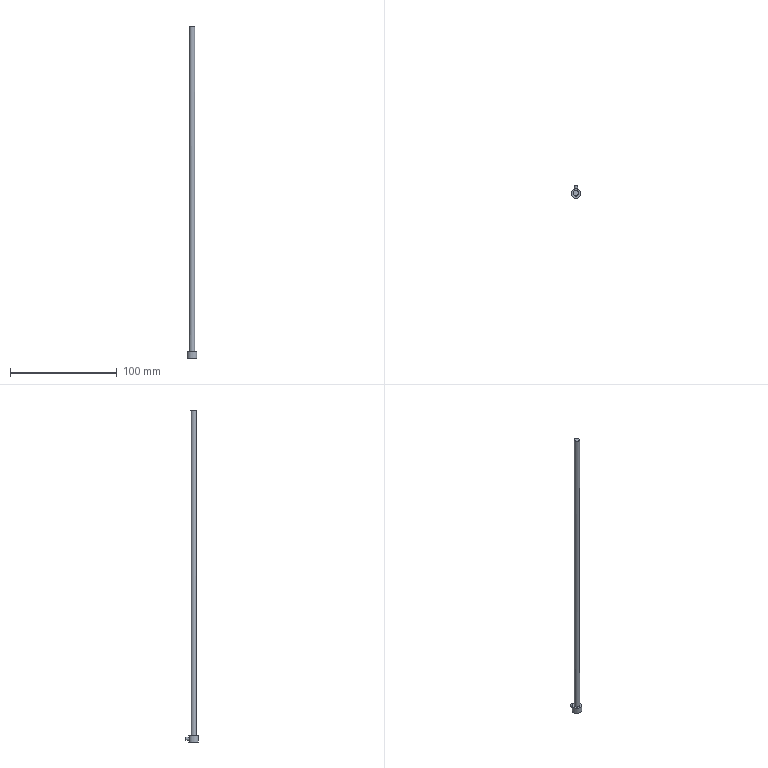Part | STEP file | E105-29-315 | 1 solid | 8 faces | box 9 x 12 x 311.151 mm | volume 6392 mm3 | cylinder 3 | plane 3 | spline 1 | cone 1 | commonest cylinder face diameters 3 x1 5 x1 9 x1
STEP:
#1=CARTESIAN_POINT('',(0.,0.,0.));
#2=DIRECTION('',(0.,0.,1.));
#3=DIRECTION('',(1.,0.,0.));
#4=AXIS2_PLACEMENT_3D('',#1,#2,#3);
#5=CARTESIAN_POINT('',(2.494,-0.1722,310.881));
#6=VERTEX_POINT('',#5);
#7=CARTESIAN_POINT('',(-2.5,0.,311.113));
#8=VERTEX_POINT('',#7);
#9=CARTESIAN_POINT('',(2.494,-0.1722,310.881));
#10=CARTESIAN_POINT('',(2.475,-0.4516,310.892));
#11=CARTESIAN_POINT('',(2.407,-0.7315,310.907));
#12=CARTESIAN_POINT('',(2.296,-0.9886,310.923));
#13=CARTESIAN_POINT('',(2.186,-1.246,310.939));
#14=CARTESIAN_POINT('',(2.029,-1.487,310.957));
#15=CARTESIAN_POINT('',(1.839,-1.693,310.975));
#16=CARTESIAN_POINT('',(1.65,-1.899,310.994));
#17=CARTESIAN_POINT('',(1.422,-2.075,311.013));
#18=CARTESIAN_POINT('',(1.174,-2.207,311.031));
#19=CARTESIAN_POINT('',(0.9268,-2.339,311.049));
#20=CARTESIAN_POINT('',(0.653,-2.429,311.066));
#21=CARTESIAN_POINT('',(0.3756,-2.472,311.081));
#22=CARTESIAN_POINT('',(0.09849,-2.514,311.097));
#23=CARTESIAN_POINT('',(-0.1899,-2.509,311.11));
#24=CARTESIAN_POINT('',(-0.4655,-2.456,311.121));
#25=CARTESIAN_POINT('',(-0.7405,-2.404,311.131));
#26=CARTESIAN_POINT('',(-1.01,-2.304,311.14));
#27=CARTESIAN_POINT('',(-1.253,-2.163,311.145));
#28=CARTESIAN_POINT('',(-1.495,-2.023,311.15));
#29=CARTESIAN_POINT('',(-1.716,-1.84,311.152));
#30=CARTESIAN_POINT('',(-1.898,-1.627,311.151));
#31=CARTESIAN_POINT('',(-2.08,-1.415,311.15));
#32=CARTESIAN_POINT('',(-2.227,-1.169,311.147));
#33=CARTESIAN_POINT('',(-2.329,-0.909,311.141));
#34=CARTESIAN_POINT('',(-2.43,-0.6487,311.135));
#35=CARTESIAN_POINT('',(-2.489,-0.3675,311.126));
#36=CARTESIAN_POINT('',(-2.498,-0.08843,311.116));
#37=CARTESIAN_POINT('',(-2.508,0.191,311.106));
#38=CARTESIAN_POINT('',(-2.47,0.4758,311.094));
#39=CARTESIAN_POINT('',(-2.387,0.7427,311.08));
#40=CARTESIAN_POINT('',(-2.304,1.01,311.067));
#41=CARTESIAN_POINT('',(-2.174,1.266,311.052));
#42=CARTESIAN_POINT('',(-2.007,1.491,311.037));
#43=CARTESIAN_POINT('',(-1.84,1.716,311.022));
#44=CARTESIAN_POINT('',(-1.632,1.915,311.006));
#45=CARTESIAN_POINT('',(-1.4,2.072,310.99));
#46=CARTESIAN_POINT('',(-1.167,2.228,310.974));
#47=CARTESIAN_POINT('',(-0.9049,2.347,310.958));
#48=CARTESIAN_POINT('',(-0.6337,2.418,310.943));
#49=CARTESIAN_POINT('',(-0.3626,2.489,310.928));
#50=CARTESIAN_POINT('',(-0.07546,2.515,310.914));
#51=CARTESIAN_POINT('',(0.204,2.492,310.901));
#52=CARTESIAN_POINT('',(0.4832,2.469,310.889));
#53=CARTESIAN_POINT('',(0.7624,2.397,310.877));
#54=CARTESIAN_POINT('',(1.018,2.283,310.868));
#55=CARTESIAN_POINT('',(1.274,2.169,310.859));
#56=CARTESIAN_POINT('',(1.514,2.009,310.853));
#57=CARTESIAN_POINT('',(1.717,1.817,310.849));
#58=CARTESIAN_POINT('',(1.92,1.625,310.845));
#59=CARTESIAN_POINT('',(2.093,1.395,310.844));
#60=CARTESIAN_POINT('',(2.221,1.147,310.846));
#61=CARTESIAN_POINT('',(2.349,0.8988,310.848));
#62=CARTESIAN_POINT('',(2.437,0.6252,310.854));
#63=CARTESIAN_POINT('',(2.476,0.3488,310.862));
#64=CARTESIAN_POINT('',(2.5,0.1767,310.867));
#65=CARTESIAN_POINT('',(2.506,0.001161,310.873));
#66=CARTESIAN_POINT('',(2.494,-0.1722,310.881));
#67=B_SPLINE_CURVE_WITH_KNOTS('',3,(#9,#10,#11,#12,#13,#14,#15,#16,#17,#18,#19,#20,#21,#22,#23,#24,#25,#26,#27,#28,#29,#30,#31,#32,#33,#34,#35,#36,#37,#38,#39,#40,#41,#42,#43,#44,#45,#46,#47,#48,#49,#50,#51,#52,#53,#54,#55,#56,#57,#58,#59,#60,#61,#62,#63,#64,#65,#66),.UNSPECIFIED.,.T.,.F.,(1,3,3,3,3,3,3,3,3,3,3,3,3,3,3,3,3,3,3,3,3,1),(-0.03305,0.,0.05377,0.1075,0.1614,0.2153,0.2691,0.3228,0.3764,0.43,0.4835,0.5372,0.5909,0.6447,0.6985,0.7523,0.8061,0.8598,0.9134,0.967,1.,1.054),.UNSPECIFIED.);
#68=CARTESIAN_POINT('',(0.,0.,106.));
#69=DIRECTION('',(0.,0.,-1.));
#70=DIRECTION('',(-1.,0.,0.));
#71=AXIS2_PLACEMENT_3D('',#68,#69,#70);
#72=CYLINDRICAL_SURFACE('',#71,2.5);
#73=CARTESIAN_POINT('',(3.211,-204.881));
#74=CARTESIAN_POINT('',(3.234,-204.883));
#75=CARTESIAN_POINT('',(3.282,-204.888));
#76=CARTESIAN_POINT('',(3.353,-204.897));
#77=CARTESIAN_POINT('',(3.425,-204.906));
#78=CARTESIAN_POINT('',(3.496,-204.916));
#79=CARTESIAN_POINT('',(3.567,-204.926));
#80=CARTESIAN_POINT('',(3.638,-204.936));
#81=CARTESIAN_POINT('',(3.71,-204.947));
#82=CARTESIAN_POINT('',(3.781,-204.958));
#83=CARTESIAN_POINT('',(3.853,-204.97));
#84=CARTESIAN_POINT('',(3.924,-204.981));
#85=CARTESIAN_POINT('',(3.995,-204.993));
#86=CARTESIAN_POINT('',(4.067,-205.005));
#87=CARTESIAN_POINT('',(4.138,-205.017));
#88=CARTESIAN_POINT('',(4.209,-205.028));
#89=CARTESIAN_POINT('',(4.28,-205.04));
#90=CARTESIAN_POINT('',(4.352,-205.051));
#91=CARTESIAN_POINT('',(4.423,-205.062));
#92=CARTESIAN_POINT('',(4.495,-205.072));
#93=CARTESIAN_POINT('',(4.566,-205.082));
#94=CARTESIAN_POINT('',(4.637,-205.091));
#95=CARTESIAN_POINT('',(4.708,-205.1));
#96=CARTESIAN_POINT('',(4.78,-205.108));
#97=CARTESIAN_POINT('',(4.851,-205.116));
#98=CARTESIAN_POINT('',(4.922,-205.123));
#99=CARTESIAN_POINT('',(4.994,-205.129));
#100=CARTESIAN_POINT('',(5.065,-205.135));
#101=CARTESIAN_POINT('',(5.137,-205.139));
#102=CARTESIAN_POINT('',(5.208,-205.143));
#103=CARTESIAN_POINT('',(5.279,-205.147));
#104=CARTESIAN_POINT('',(5.351,-205.149));
#105=CARTESIAN_POINT('',(5.423,-205.151));
#106=CARTESIAN_POINT('',(5.494,-205.151));
#107=CARTESIAN_POINT('',(5.566,-205.151));
#108=CARTESIAN_POINT('',(5.637,-205.151));
#109=CARTESIAN_POINT('',(5.708,-205.149));
#110=CARTESIAN_POINT('',(5.78,-205.147));
#111=CARTESIAN_POINT('',(5.852,-205.144));
#112=CARTESIAN_POINT('',(5.923,-205.14));
#113=CARTESIAN_POINT('',(5.994,-205.136));
#114=CARTESIAN_POINT('',(6.066,-205.131));
#115=CARTESIAN_POINT('',(6.137,-205.126));
#116=CARTESIAN_POINT('',(6.209,-205.12));
#117=CARTESIAN_POINT('',(6.28,-205.113));
#118=CARTESIAN_POINT('',(6.351,-205.106));
#119=CARTESIAN_POINT('',(6.423,-205.099));
#120=CARTESIAN_POINT('',(6.494,-205.091));
#121=CARTESIAN_POINT('',(6.566,-205.083));
#122=CARTESIAN_POINT('',(6.637,-205.074));
#123=CARTESIAN_POINT('',(6.708,-205.065));
#124=CARTESIAN_POINT('',(6.78,-205.056));
#125=CARTESIAN_POINT('',(6.851,-205.047));
#126=CARTESIAN_POINT('',(6.922,-205.037));
#127=CARTESIAN_POINT('',(6.993,-205.027));
#128=CARTESIAN_POINT('',(7.065,-205.017));
#129=CARTESIAN_POINT('',(7.136,-205.007));
#130=CARTESIAN_POINT('',(7.208,-204.997));
#131=CARTESIAN_POINT('',(7.279,-204.987));
#132=CARTESIAN_POINT('',(7.35,-204.977));
#133=CARTESIAN_POINT('',(7.422,-204.967));
#134=CARTESIAN_POINT('',(7.493,-204.958));
#135=CARTESIAN_POINT('',(7.564,-204.948));
#136=CARTESIAN_POINT('',(7.635,-204.938));
#137=CARTESIAN_POINT('',(7.707,-204.929));
#138=CARTESIAN_POINT('',(7.778,-204.92));
#139=CARTESIAN_POINT('',(7.85,-204.911));
#140=CARTESIAN_POINT('',(7.921,-204.903));
#141=CARTESIAN_POINT('',(7.992,-204.895));
#142=CARTESIAN_POINT('',(8.064,-204.887));
#143=CARTESIAN_POINT('',(8.135,-204.88));
#144=CARTESIAN_POINT('',(8.207,-204.874));
#145=CARTESIAN_POINT('',(8.278,-204.868));
#146=CARTESIAN_POINT('',(8.349,-204.863));
#147=CARTESIAN_POINT('',(8.421,-204.858));
#148=CARTESIAN_POINT('',(8.492,-204.854));
#149=CARTESIAN_POINT('',(8.564,-204.85));
#150=CARTESIAN_POINT('',(8.635,-204.848));
#151=CARTESIAN_POINT('',(8.706,-204.846));
#152=CARTESIAN_POINT('',(8.778,-204.845));
#153=CARTESIAN_POINT('',(8.85,-204.845));
#154=CARTESIAN_POINT('',(8.921,-204.846));
#155=CARTESIAN_POINT('',(8.992,-204.847));
#156=CARTESIAN_POINT('',(9.064,-204.849));
#157=CARTESIAN_POINT('',(9.135,-204.853));
#158=CARTESIAN_POINT('',(9.207,-204.857));
#159=CARTESIAN_POINT('',(9.278,-204.861));
#160=CARTESIAN_POINT('',(9.35,-204.867));
#161=CARTESIAN_POINT('',(9.422,-204.873));
#162=CARTESIAN_POINT('',(9.47,-204.878));
#163=CARTESIAN_POINT('',(9.494,-204.881));
#164=B_SPLINE_CURVE_WITH_KNOTS('',3,(#73,#74,#75,#76,#77,#78,#79,#80,#81,#82,#83,#84,#85,#86,#87,#88,#89,#90,#91,#92,#93,#94,#95,#96,#97,#98,#99,#100,#101,#102,#103,#104,#105,#106,#107,#108,#109,#110,#111,#112,#113,#114,#115,#116,#117,#118,#119,#120,#121,#122,#123,#124,#125,#126,#127,#128,#129,#130,#131,#132,#133,#134,#135,#136,#137,#138,#139,#140,#141,#142,#143,#144,#145,#146,#147,#148,#149,#150,#151,#152,#153,#154,#155,#156,#157,#158,#159,#160,#161,#162,#163),.UNSPECIFIED.,.F.,.F.,(4,1,1,1,1,1,1,1,1,1,1,1,1,1,1,1,1,1,1,1,1,1,1,1,1,1,1,1,1,1,1,1,1,1,1,1,1,1,1,1,1,1,1,1,1,1,1,1,1,1,1,1,1,1,1,1,1,1,1,1,1,1,1,1,1,1,1,1,1,1,1,1,1,1,1,1,1,1,1,1,1,1,1,1,1,1,1,1,4),(0.,0.01136,0.02273,0.03409,0.04545,0.05682,0.06818,0.07955,0.09091,0.1023,0.1136,0.125,0.1364,0.1477,0.1591,0.1705,0.1818,0.1932,0.2045,0.2159,0.2273,0.2386,0.25,0.2614,0.2727,0.2841,0.2955,0.3068,0.3182,0.3295,0.3409,0.3523,0.3636,0.375,0.3864,0.3977,0.4091,0.4205,0.4318,0.4432,0.4545,0.4659,0.4773,0.4886,0.5,0.5114,0.5227,0.5341,0.5455,0.5568,0.5682,0.5795,0.5909,0.6023,0.6136,0.625,0.6364,0.6477,0.6591,0.6705,0.6818,0.6932,0.7045,0.7159,0.7273,0.7386,0.75,0.7614,0.7727,0.7841,0.7955,0.8068,0.8182,0.8295,0.8409,0.8523,0.8636,0.875,0.8864,0.8977,0.9091,0.9205,0.9318,0.9432,0.9545,0.9659,0.9773,0.9886,1.),.QUASI_UNIFORM_KNOTS.);
#165=(GEOMETRIC_REPRESENTATION_CONTEXT(2)PARAMETRIC_REPRESENTATION_CONTEXT()REPRESENTATION_CONTEXT('',''));
#166=DEFINITIONAL_REPRESENTATION('',(#164),#165);
#167=PCURVE('',#72,#166);
#168=CARTESIAN_POINT('',(-12.782,-3.331,311.416));
#169=CARTESIAN_POINT('',(-7.05,-3.329,311.438));
#170=CARTESIAN_POINT('',(-1.256,-3.327,311.257));
#171=CARTESIAN_POINT('',(4.609,-3.325,310.869));
#172=CARTESIAN_POINT('',(-12.796,-0.9979,311.327));
#173=CARTESIAN_POINT('',(-7.066,-0.9958,311.349));
#174=CARTESIAN_POINT('',(-1.274,-0.9937,311.169));
#175=CARTESIAN_POINT('',(4.59,-0.9916,310.782));
#176=CARTESIAN_POINT('',(-12.81,1.335,311.238));
#177=CARTESIAN_POINT('',(-7.082,1.337,311.261));
#178=CARTESIAN_POINT('',(-1.292,1.339,311.081));
#179=CARTESIAN_POINT('',(4.57,1.342,310.695));
#180=CARTESIAN_POINT('',(-12.825,3.668,311.148));
#181=CARTESIAN_POINT('',(-7.099,3.671,311.172));
#182=CARTESIAN_POINT('',(-1.31,3.673,310.993));
#183=CARTESIAN_POINT('',(4.55,3.675,310.608));
#184=B_SPLINE_SURFACE_WITH_KNOTS('',3,3,((#168,#169,#170,#171),(#172,#173,#174,#175),(#176,#177,#178,#179),(#180,#181,#182,#183)),.UNSPECIFIED.,.F.,.F.,.F.,(4,4),(4,4),(0.,1.),(0.,1.),.PIECEWISE_BEZIER_KNOTS.);
#185=CARTESIAN_POINT('',(0.4505,0.8811));
#186=CARTESIAN_POINT('',(0.4423,0.8808));
#187=CARTESIAN_POINT('',(0.4257,0.8801));
#188=CARTESIAN_POINT('',(0.4011,0.8783));
#189=CARTESIAN_POINT('',(0.3768,0.8758));
#190=CARTESIAN_POINT('',(0.3531,0.8726));
#191=CARTESIAN_POINT('',(0.33,0.8689));
#192=CARTESIAN_POINT('',(0.3077,0.8644));
#193=CARTESIAN_POINT('',(0.286,0.8594));
#194=CARTESIAN_POINT('',(0.2653,0.8537));
#195=CARTESIAN_POINT('',(0.2456,0.8475));
#196=CARTESIAN_POINT('',(0.2271,0.8409));
#197=CARTESIAN_POINT('',(0.2098,0.8337));
#198=CARTESIAN_POINT('',(0.1938,0.826));
#199=CARTESIAN_POINT('',(0.1791,0.8179));
#200=CARTESIAN_POINT('',(0.1658,0.8094));
#201=CARTESIAN_POINT('',(0.1541,0.8006));
#202=CARTESIAN_POINT('',(0.144,0.7914));
#203=CARTESIAN_POINT('',(0.1354,0.782));
#204=CARTESIAN_POINT('',(0.1285,0.7724));
#205=CARTESIAN_POINT('',(0.1233,0.7626));
#206=CARTESIAN_POINT('',(0.1198,0.7528));
#207=CARTESIAN_POINT('',(0.118,0.7428));
#208=CARTESIAN_POINT('',(0.118,0.7328));
#209=CARTESIAN_POINT('',(0.1197,0.7228));
#210=CARTESIAN_POINT('',(0.1231,0.7129));
#211=CARTESIAN_POINT('',(0.1283,0.7032));
#212=CARTESIAN_POINT('',(0.1352,0.6936));
#213=CARTESIAN_POINT('',(0.1437,0.6842));
#214=CARTESIAN_POINT('',(0.1539,0.675));
#215=CARTESIAN_POINT('',(0.1655,0.6663));
#216=CARTESIAN_POINT('',(0.1787,0.6578));
#217=CARTESIAN_POINT('',(0.1934,0.6497));
#218=CARTESIAN_POINT('',(0.2095,0.6421));
#219=CARTESIAN_POINT('',(0.2269,0.6349));
#220=CARTESIAN_POINT('',(0.2454,0.6283));
#221=CARTESIAN_POINT('',(0.265,0.6222));
#222=CARTESIAN_POINT('',(0.2858,0.6166));
#223=CARTESIAN_POINT('',(0.3075,0.6116));
#224=CARTESIAN_POINT('',(0.3299,0.6073));
#225=CARTESIAN_POINT('',(0.353,0.6036));
#226=CARTESIAN_POINT('',(0.3767,0.6006));
#227=CARTESIAN_POINT('',(0.401,0.5982));
#228=CARTESIAN_POINT('',(0.4257,0.5966));
#229=CARTESIAN_POINT('',(0.4505,0.5956));
#230=CARTESIAN_POINT('',(0.4671,0.5954));
#231=CARTESIAN_POINT('',(0.4754,0.5954));
#232=B_SPLINE_CURVE_WITH_KNOTS('',3,(#185,#186,#187,#188,#189,#190,#191,#192,#193,#194,#195,#196,#197,#198,#199,#200,#201,#202,#203,#204,#205,#206,#207,#208,#209,#210,#211,#212,#213,#214,#215,#216,#217,#218,#219,#220,#221,#222,#223,#224,#225,#226,#227,#228,#229,#230,#231),.UNSPECIFIED.,.F.,.F.,(4,1,1,1,1,1,1,1,1,1,1,1,1,1,1,1,1,1,1,1,1,1,1,1,1,1,1,1,1,1,1,1,1,1,1,1,1,1,1,1,1,1,1,1,4),(0.,0.01112,0.02224,0.03335,0.04447,0.05559,0.06671,0.07783,0.08894,0.1001,0.1112,0.1223,0.1334,0.1445,0.1557,0.1668,0.1779,0.189,0.2001,0.2112,0.2224,0.2335,0.2446,0.2557,0.2668,0.2779,0.2891,0.3002,0.3113,0.3224,0.3335,0.3447,0.3558,0.3669,0.378,0.3891,0.4002,0.4114,0.4225,0.4336,0.4447,0.4558,0.467,0.4781,0.4892),.QUASI_UNIFORM_KNOTS.);
#233=(GEOMETRIC_REPRESENTATION_CONTEXT(2)PARAMETRIC_REPRESENTATION_CONTEXT()REPRESENTATION_CONTEXT('',''));
#234=DEFINITIONAL_REPRESENTATION('',(#232),#233);
#235=PCURVE('',#184,#234);
#236=SURFACE_CURVE('',#67,(#167,#235),.PCURVE_S1.);
#237=EDGE_CURVE('',#6,#8,#236,.T.);
#238=ORIENTED_EDGE('',*,*,#237,.T.);
#239=CARTESIAN_POINT('',(-2.5,0.,6.));
#240=VERTEX_POINT('',#239);
#241=CARTESIAN_POINT('',(-2.5,0.,311.113));
#242=CARTESIAN_POINT('',(-2.5,0.,6.));
#243=B_SPLINE_CURVE_WITH_KNOTS('',1,(#241,#242),.UNSPECIFIED.,.F.,.F.,(2,2),(-205.113,100.),.PIECEWISE_BEZIER_KNOTS.);
#244=CARTESIAN_POINT('',(6.283,0.));
#245=DIRECTION('',(0.,1.));
#246=VECTOR('',#245,1.);
#247=LINE('',#244,#246);
#248=(GEOMETRIC_REPRESENTATION_CONTEXT(2)PARAMETRIC_REPRESENTATION_CONTEXT()REPRESENTATION_CONTEXT('',''));
#249=DEFINITIONAL_REPRESENTATION('',(#247),#248);
#250=PCURVE('',#72,#249);
#251=CARTESIAN_POINT('',(0.,0.));
#252=DIRECTION('',(0.,1.));
#253=VECTOR('',#252,1.);
#254=LINE('',#251,#253);
#255=(GEOMETRIC_REPRESENTATION_CONTEXT(2)PARAMETRIC_REPRESENTATION_CONTEXT()REPRESENTATION_CONTEXT('',''));
#256=DEFINITIONAL_REPRESENTATION('',(#254),#255);
#257=PCURVE('',#72,#256);
#258=SEAM_CURVE('',#243,(#250,#257),.PCURVE_S1.);
#259=EDGE_CURVE('',#8,#240,#258,.T.);
#260=ORIENTED_EDGE('',*,*,#259,.T.);
#261=CARTESIAN_POINT('',(0.,0.,6.));
#262=DIRECTION('',(0.,0.,-1.));
#263=DIRECTION('',(-1.,0.,0.));
#264=AXIS2_PLACEMENT_3D('',#261,#262,#263);
#265=CIRCLE('',#264,2.5);
#266=CARTESIAN_POINT('',(0.,100.));
#267=DIRECTION('',(1.,0.));
#268=VECTOR('',#267,1.);
#269=LINE('',#266,#268);
#270=(GEOMETRIC_REPRESENTATION_CONTEXT(2)PARAMETRIC_REPRESENTATION_CONTEXT()REPRESENTATION_CONTEXT('',''));
#271=DEFINITIONAL_REPRESENTATION('',(#269),#270);
#272=PCURVE('',#72,#271);
#273=CARTESIAN_POINT('',(0.,0.,6.));
#274=DIRECTION('',(0.,0.,-1.));
#275=DIRECTION('',(1.,0.,0.));
#276=AXIS2_PLACEMENT_3D('',#273,#274,#275);
#277=PLANE('',#276);
#278=CARTESIAN_POINT('',(0.,0.));
#279=DIRECTION('',(-1.,0.));
#280=AXIS2_PLACEMENT_2D('',#278,#279);
#281=CIRCLE('',#280,2.5);
#282=(GEOMETRIC_REPRESENTATION_CONTEXT(2)PARAMETRIC_REPRESENTATION_CONTEXT()REPRESENTATION_CONTEXT('',''));
#283=DEFINITIONAL_REPRESENTATION('',(#281),#282);
#284=PCURVE('',#277,#283);
#285=SURFACE_CURVE('',#265,(#272,#284),.PCURVE_S1.);
#286=EDGE_CURVE('',#240,#240,#285,.T.);
#287=ORIENTED_EDGE('',*,*,#286,.F.);
#288=ORIENTED_EDGE('',*,*,#259,.F.);
#289=CARTESIAN_POINT('',(2.494,-0.1722,310.881));
#290=CARTESIAN_POINT('',(2.475,-0.4516,310.892));
#291=CARTESIAN_POINT('',(2.407,-0.7315,310.907));
#292=CARTESIAN_POINT('',(2.296,-0.9886,310.923));
#293=CARTESIAN_POINT('',(2.186,-1.246,310.939));
#294=CARTESIAN_POINT('',(2.029,-1.487,310.957));
#295=CARTESIAN_POINT('',(1.839,-1.693,310.975));
#296=CARTESIAN_POINT('',(1.65,-1.899,310.994));
#297=CARTESIAN_POINT('',(1.422,-2.075,311.013));
#298=CARTESIAN_POINT('',(1.174,-2.207,311.031));
#299=CARTESIAN_POINT('',(0.9268,-2.339,311.049));
#300=CARTESIAN_POINT('',(0.653,-2.429,311.066));
#301=CARTESIAN_POINT('',(0.3756,-2.472,311.081));
#302=CARTESIAN_POINT('',(0.09849,-2.514,311.097));
#303=CARTESIAN_POINT('',(-0.1899,-2.509,311.11));
#304=CARTESIAN_POINT('',(-0.4655,-2.456,311.121));
#305=CARTESIAN_POINT('',(-0.7405,-2.404,311.131));
#306=CARTESIAN_POINT('',(-1.01,-2.304,311.14));
#307=CARTESIAN_POINT('',(-1.253,-2.163,311.145));
#308=CARTESIAN_POINT('',(-1.495,-2.023,311.15));
#309=CARTESIAN_POINT('',(-1.716,-1.84,311.152));
#310=CARTESIAN_POINT('',(-1.898,-1.627,311.151));
#311=CARTESIAN_POINT('',(-2.08,-1.415,311.15));
#312=CARTESIAN_POINT('',(-2.227,-1.169,311.147));
#313=CARTESIAN_POINT('',(-2.329,-0.909,311.141));
#314=CARTESIAN_POINT('',(-2.43,-0.6487,311.135));
#315=CARTESIAN_POINT('',(-2.489,-0.3675,311.126));
#316=CARTESIAN_POINT('',(-2.498,-0.08843,311.116));
#317=CARTESIAN_POINT('',(-2.508,0.191,311.106));
#318=CARTESIAN_POINT('',(-2.47,0.4758,311.094));
#319=CARTESIAN_POINT('',(-2.387,0.7427,311.08));
#320=CARTESIAN_POINT('',(-2.304,1.01,311.067));
#321=CARTESIAN_POINT('',(-2.174,1.266,311.052));
#322=CARTESIAN_POINT('',(-2.007,1.491,311.037));
#323=CARTESIAN_POINT('',(-1.84,1.716,311.022));
#324=CARTESIAN_POINT('',(-1.632,1.915,311.006));
#325=CARTESIAN_POINT('',(-1.4,2.072,310.99));
#326=CARTESIAN_POINT('',(-1.167,2.228,310.974));
#327=CARTESIAN_POINT('',(-0.9049,2.347,310.958));
#328=CARTESIAN_POINT('',(-0.6337,2.418,310.943));
#329=CARTESIAN_POINT('',(-0.3626,2.489,310.928));
#330=CARTESIAN_POINT('',(-0.07546,2.515,310.914));
#331=CARTESIAN_POINT('',(0.204,2.492,310.901));
#332=CARTESIAN_POINT('',(0.4832,2.469,310.889));
#333=CARTESIAN_POINT('',(0.7624,2.397,310.877));
#334=CARTESIAN_POINT('',(1.018,2.283,310.868));
#335=CARTESIAN_POINT('',(1.274,2.169,310.859));
#336=CARTESIAN_POINT('',(1.514,2.009,310.853));
#337=CARTESIAN_POINT('',(1.717,1.817,310.849));
#338=CARTESIAN_POINT('',(1.92,1.625,310.845));
#339=CARTESIAN_POINT('',(2.093,1.395,310.844));
#340=CARTESIAN_POINT('',(2.221,1.147,310.846));
#341=CARTESIAN_POINT('',(2.349,0.8988,310.848));
#342=CARTESIAN_POINT('',(2.437,0.6252,310.854));
#343=CARTESIAN_POINT('',(2.476,0.3488,310.862));
#344=CARTESIAN_POINT('',(2.5,0.1767,310.867));
#345=CARTESIAN_POINT('',(2.506,0.001161,310.873));
#346=CARTESIAN_POINT('',(2.494,-0.1722,310.881));
#347=B_SPLINE_CURVE_WITH_KNOTS('',3,(#289,#290,#291,#292,#293,#294,#295,#296,#297,#298,#299,#300,#301,#302,#303,#304,#305,#306,#307,#308,#309,#310,#311,#312,#313,#314,#315,#316,#317,#318,#319,#320,#321,#322,#323,#324,#325,#326,#327,#328,#329,#330,#331,#332,#333,#334,#335,#336,#337,#338,#339,#340,#341,#342,#343,#344,#345,#346),.UNSPECIFIED.,.T.,.F.,(1,3,3,3,3,3,3,3,3,3,3,3,3,3,3,3,3,3,3,3,3,1),(-0.03305,0.,0.05377,0.1075,0.1614,0.2153,0.2691,0.3228,0.3764,0.43,0.4835,0.5372,0.5909,0.6447,0.6985,0.7523,0.8061,0.8598,0.9134,0.967,1.,1.054),.UNSPECIFIED.);
#348=CARTESIAN_POINT('',(-3.073,-204.881));
#349=CARTESIAN_POINT('',(-3.049,-204.883));
#350=CARTESIAN_POINT('',(-3.001,-204.888));
#351=CARTESIAN_POINT('',(-2.93,-204.897));
#352=CARTESIAN_POINT('',(-2.858,-204.906));
#353=CARTESIAN_POINT('',(-2.787,-204.916));
#354=CARTESIAN_POINT('',(-2.716,-204.926));
#355=CARTESIAN_POINT('',(-2.645,-204.936));
#356=CARTESIAN_POINT('',(-2.573,-204.947));
#357=CARTESIAN_POINT('',(-2.502,-204.958));
#358=CARTESIAN_POINT('',(-2.43,-204.97));
#359=CARTESIAN_POINT('',(-2.359,-204.981));
#360=CARTESIAN_POINT('',(-2.288,-204.993));
#361=CARTESIAN_POINT('',(-2.217,-205.005));
#362=CARTESIAN_POINT('',(-2.145,-205.017));
#363=CARTESIAN_POINT('',(-2.074,-205.028));
#364=CARTESIAN_POINT('',(-2.003,-205.04));
#365=CARTESIAN_POINT('',(-1.932,-205.051));
#366=CARTESIAN_POINT('',(-1.86,-205.062));
#367=CARTESIAN_POINT('',(-1.789,-205.072));
#368=CARTESIAN_POINT('',(-1.718,-205.082));
#369=CARTESIAN_POINT('',(-1.646,-205.091));
#370=CARTESIAN_POINT('',(-1.575,-205.1));
#371=CARTESIAN_POINT('',(-1.503,-205.108));
#372=CARTESIAN_POINT('',(-1.432,-205.116));
#373=CARTESIAN_POINT('',(-1.361,-205.123));
#374=CARTESIAN_POINT('',(-1.289,-205.129));
#375=CARTESIAN_POINT('',(-1.218,-205.135));
#376=CARTESIAN_POINT('',(-1.146,-205.139));
#377=CARTESIAN_POINT('',(-1.075,-205.143));
#378=CARTESIAN_POINT('',(-1.004,-205.147));
#379=CARTESIAN_POINT('',(-0.9322,-205.149));
#380=CARTESIAN_POINT('',(-0.8606,-205.151));
#381=CARTESIAN_POINT('',(-0.7889,-205.151));
#382=CARTESIAN_POINT('',(-0.7176,-205.151));
#383=CARTESIAN_POINT('',(-0.6465,-205.151));
#384=CARTESIAN_POINT('',(-0.5749,-205.149));
#385=CARTESIAN_POINT('',(-0.5033,-205.147));
#386=CARTESIAN_POINT('',(-0.4317,-205.144));
#387=CARTESIAN_POINT('',(-0.3605,-205.14));
#388=CARTESIAN_POINT('',(-0.2892,-205.136));
#389=CARTESIAN_POINT('',(-0.2176,-205.131));
#390=CARTESIAN_POINT('',(-0.146,-205.126));
#391=CARTESIAN_POINT('',(-0.07455,-205.12));
#392=CARTESIAN_POINT('',(-0.003524,-205.113));
#393=CARTESIAN_POINT('',(0.06789,-205.106));
#394=CARTESIAN_POINT('',(0.1395,-205.099));
#395=CARTESIAN_POINT('',(0.211,-205.091));
#396=CARTESIAN_POINT('',(0.2823,-205.083));
#397=CARTESIAN_POINT('',(0.3534,-205.074));
#398=CARTESIAN_POINT('',(0.4248,-205.065));
#399=CARTESIAN_POINT('',(0.4964,-205.056));
#400=CARTESIAN_POINT('',(0.5679,-205.047));
#401=CARTESIAN_POINT('',(0.639,-205.037));
#402=CARTESIAN_POINT('',(0.7101,-205.027));
#403=CARTESIAN_POINT('',(0.7816,-205.017));
#404=CARTESIAN_POINT('',(0.8532,-205.007));
#405=CARTESIAN_POINT('',(0.9246,-204.997));
#406=CARTESIAN_POINT('',(0.9956,-204.987));
#407=CARTESIAN_POINT('',(1.067,-204.977));
#408=CARTESIAN_POINT('',(1.138,-204.967));
#409=CARTESIAN_POINT('',(1.21,-204.958));
#410=CARTESIAN_POINT('',(1.281,-204.948));
#411=CARTESIAN_POINT('',(1.352,-204.938));
#412=CARTESIAN_POINT('',(1.424,-204.929));
#413=CARTESIAN_POINT('',(1.495,-204.92));
#414=CARTESIAN_POINT('',(1.567,-204.911));
#415=CARTESIAN_POINT('',(1.638,-204.903));
#416=CARTESIAN_POINT('',(1.709,-204.895));
#417=CARTESIAN_POINT('',(1.781,-204.887));
#418=CARTESIAN_POINT('',(1.852,-204.88));
#419=CARTESIAN_POINT('',(1.924,-204.874));
#420=CARTESIAN_POINT('',(1.995,-204.868));
#421=CARTESIAN_POINT('',(2.066,-204.863));
#422=CARTESIAN_POINT('',(2.138,-204.858));
#423=CARTESIAN_POINT('',(2.209,-204.854));
#424=CARTESIAN_POINT('',(2.281,-204.85));
#425=CARTESIAN_POINT('',(2.352,-204.848));
#426=CARTESIAN_POINT('',(2.423,-204.846));
#427=CARTESIAN_POINT('',(2.495,-204.845));
#428=CARTESIAN_POINT('',(2.567,-204.845));
#429=CARTESIAN_POINT('',(2.638,-204.846));
#430=CARTESIAN_POINT('',(2.709,-204.847));
#431=CARTESIAN_POINT('',(2.781,-204.849));
#432=CARTESIAN_POINT('',(2.852,-204.853));
#433=CARTESIAN_POINT('',(2.924,-204.857));
#434=CARTESIAN_POINT('',(2.995,-204.861));
#435=CARTESIAN_POINT('',(3.067,-204.867));
#436=CARTESIAN_POINT('',(3.139,-204.873));
#437=CARTESIAN_POINT('',(3.187,-204.878));
#438=CARTESIAN_POINT('',(3.211,-204.881));
#439=B_SPLINE_CURVE_WITH_KNOTS('',3,(#348,#349,#350,#351,#352,#353,#354,#355,#356,#357,#358,#359,#360,#361,#362,#363,#364,#365,#366,#367,#368,#369,#370,#371,#372,#373,#374,#375,#376,#377,#378,#379,#380,#381,#382,#383,#384,#385,#386,#387,#388,#389,#390,#391,#392,#393,#394,#395,#396,#397,#398,#399,#400,#401,#402,#403,#404,#405,#406,#407,#408,#409,#410,#411,#412,#413,#414,#415,#416,#417,#418,#419,#420,#421,#422,#423,#424,#425,#426,#427,#428,#429,#430,#431,#432,#433,#434,#435,#436,#437,#438),.UNSPECIFIED.,.F.,.F.,(4,1,1,1,1,1,1,1,1,1,1,1,1,1,1,1,1,1,1,1,1,1,1,1,1,1,1,1,1,1,1,1,1,1,1,1,1,1,1,1,1,1,1,1,1,1,1,1,1,1,1,1,1,1,1,1,1,1,1,1,1,1,1,1,1,1,1,1,1,1,1,1,1,1,1,1,1,1,1,1,1,1,1,1,1,1,1,1,4),(0.,0.01136,0.02273,0.03409,0.04545,0.05682,0.06818,0.07955,0.09091,0.1023,0.1136,0.125,0.1364,0.1477,0.1591,0.1705,0.1818,0.1932,0.2045,0.2159,0.2273,0.2386,0.25,0.2614,0.2727,0.2841,0.2955,0.3068,0.3182,0.3295,0.3409,0.3523,0.3636,0.375,0.3864,0.3977,0.4091,0.4205,0.4318,0.4432,0.4545,0.4659,0.4773,0.4886,0.5,0.5114,0.5227,0.5341,0.5455,0.5568,0.5682,0.5795,0.5909,0.6023,0.6136,0.625,0.6364,0.6477,0.6591,0.6705,0.6818,0.6932,0.7045,0.7159,0.7273,0.7386,0.75,0.7614,0.7727,0.7841,0.7955,0.8068,0.8182,0.8295,0.8409,0.8523,0.8636,0.875,0.8864,0.8977,0.9091,0.9205,0.9318,0.9432,0.9545,0.9659,0.9773,0.9886,1.),.QUASI_UNIFORM_KNOTS.);
#440=(GEOMETRIC_REPRESENTATION_CONTEXT(2)PARAMETRIC_REPRESENTATION_CONTEXT()REPRESENTATION_CONTEXT('',''));
#441=DEFINITIONAL_REPRESENTATION('',(#439),#440);
#442=PCURVE('',#72,#441);
#443=CARTESIAN_POINT('',(0.4754,0.5954));
#444=CARTESIAN_POINT('',(0.484,0.5955));
#445=CARTESIAN_POINT('',(0.5014,0.5958));
#446=CARTESIAN_POINT('',(0.5274,0.597));
#447=CARTESIAN_POINT('',(0.5531,0.599));
#448=CARTESIAN_POINT('',(0.5782,0.6017));
#449=CARTESIAN_POINT('',(0.6028,0.6051));
#450=CARTESIAN_POINT('',(0.6268,0.6093));
#451=CARTESIAN_POINT('',(0.6501,0.6142));
#452=CARTESIAN_POINT('',(0.6724,0.6197));
#453=CARTESIAN_POINT('',(0.6935,0.6258));
#454=CARTESIAN_POINT('',(0.7135,0.6325));
#455=CARTESIAN_POINT('',(0.7323,0.6399));
#456=CARTESIAN_POINT('',(0.7497,0.6477));
#457=CARTESIAN_POINT('',(0.7657,0.656));
#458=CARTESIAN_POINT('',(0.78,0.6647));
#459=CARTESIAN_POINT('',(0.7928,0.6739));
#460=CARTESIAN_POINT('',(0.8039,0.6834));
#461=CARTESIAN_POINT('',(0.8133,0.6932));
#462=CARTESIAN_POINT('',(0.8209,0.7032));
#463=CARTESIAN_POINT('',(0.8266,0.7134));
#464=CARTESIAN_POINT('',(0.8304,0.7237));
#465=CARTESIAN_POINT('',(0.8324,0.7342));
#466=CARTESIAN_POINT('',(0.8325,0.7446));
#467=CARTESIAN_POINT('',(0.8307,0.755));
#468=CARTESIAN_POINT('',(0.827,0.7653));
#469=CARTESIAN_POINT('',(0.8214,0.7755));
#470=CARTESIAN_POINT('',(0.8139,0.7855));
#471=CARTESIAN_POINT('',(0.8047,0.7952));
#472=CARTESIAN_POINT('',(0.7938,0.8046));
#473=CARTESIAN_POINT('',(0.7811,0.8137));
#474=CARTESIAN_POINT('',(0.7667,0.8224));
#475=CARTESIAN_POINT('',(0.7509,0.8306));
#476=CARTESIAN_POINT('',(0.7336,0.8383));
#477=CARTESIAN_POINT('',(0.7149,0.8455));
#478=CARTESIAN_POINT('',(0.6949,0.8522));
#479=CARTESIAN_POINT('',(0.6737,0.8582));
#480=CARTESIAN_POINT('',(0.6515,0.8636));
#481=CARTESIAN_POINT('',(0.6285,0.8683));
#482=CARTESIAN_POINT('',(0.6045,0.8724));
#483=CARTESIAN_POINT('',(0.5798,0.8757));
#484=CARTESIAN_POINT('',(0.5545,0.8783));
#485=CARTESIAN_POINT('',(0.529,0.8802));
#486=CARTESIAN_POINT('',(0.5029,0.8813));
#487=CARTESIAN_POINT('',(0.4767,0.8816));
#488=CARTESIAN_POINT('',(0.4592,0.8813));
#489=CARTESIAN_POINT('',(0.4505,0.8811));
#490=B_SPLINE_CURVE_WITH_KNOTS('',3,(#443,#444,#445,#446,#447,#448,#449,#450,#451,#452,#453,#454,#455,#456,#457,#458,#459,#460,#461,#462,#463,#464,#465,#466,#467,#468,#469,#470,#471,#472,#473,#474,#475,#476,#477,#478,#479,#480,#481,#482,#483,#484,#485,#486,#487,#488,#489),.UNSPECIFIED.,.F.,.F.,(4,1,1,1,1,1,1,1,1,1,1,1,1,1,1,1,1,1,1,1,1,1,1,1,1,1,1,1,1,1,1,1,1,1,1,1,1,1,1,1,1,1,1,1,4),(0.4892,0.5008,0.5124,0.524,0.5356,0.5472,0.5588,0.5705,0.5821,0.5937,0.6053,0.6169,0.6285,0.6401,0.6517,0.6633,0.6749,0.6865,0.6982,0.7098,0.7214,0.733,0.7446,0.7562,0.7678,0.7794,0.791,0.8026,0.8143,0.8259,0.8375,0.8491,0.8607,0.8723,0.8839,0.8955,0.9071,0.9187,0.9303,0.942,0.9536,0.9652,0.9768,0.9884,1.),.QUASI_UNIFORM_KNOTS.);
#491=(GEOMETRIC_REPRESENTATION_CONTEXT(2)PARAMETRIC_REPRESENTATION_CONTEXT()REPRESENTATION_CONTEXT('',''));
#492=DEFINITIONAL_REPRESENTATION('',(#490),#491);
#493=PCURVE('',#184,#492);
#494=SURFACE_CURVE('',#347,(#442,#493),.PCURVE_S1.);
#495=EDGE_CURVE('',#8,#6,#494,.T.);
#496=ORIENTED_EDGE('',*,*,#495,.T.);
#497=EDGE_LOOP('',(#238,#260,#287,#288,#496));
#498=FACE_BOUND('',#497,.T.);
#499=ADVANCED_FACE('',(#498),#72,.T.);
#500=ORIENTED_EDGE('',*,*,#495,.T.);
#501=ORIENTED_EDGE('',*,*,#237,.T.);
#502=EDGE_LOOP('',(#500,#501));
#503=FACE_BOUND('',#502,.F.);
#504=ADVANCED_FACE('',(#503),#184,.F.);
#505=CARTESIAN_POINT('',(-4.5,0.,6.));
#506=VERTEX_POINT('',#505);
#507=CARTESIAN_POINT('',(0.,0.,6.));
#508=DIRECTION('',(0.,0.,-1.));
#509=DIRECTION('',(-1.,0.,0.));
#510=AXIS2_PLACEMENT_3D('',#507,#508,#509);
#511=CIRCLE('',#510,4.5);
#512=CARTESIAN_POINT('',(0.,0.));
#513=DIRECTION('',(-1.,0.));
#514=AXIS2_PLACEMENT_2D('',#512,#513);
#515=CIRCLE('',#514,4.5);
#516=(GEOMETRIC_REPRESENTATION_CONTEXT(2)PARAMETRIC_REPRESENTATION_CONTEXT()REPRESENTATION_CONTEXT('',''));
#517=DEFINITIONAL_REPRESENTATION('',(#515),#516);
#518=PCURVE('',#277,#517);
#519=CARTESIAN_POINT('',(0.,0.,-21.));
#520=DIRECTION('',(0.,0.,1.));
#521=DIRECTION('',(-1.,0.,0.));
#522=AXIS2_PLACEMENT_3D('',#519,#520,#521);
#523=CYLINDRICAL_SURFACE('',#522,4.5);
#524=CARTESIAN_POINT('',(6.283,27.));
#525=DIRECTION('',(-1.,0.));
#526=VECTOR('',#525,1.);
#527=LINE('',#524,#526);
#528=(GEOMETRIC_REPRESENTATION_CONTEXT(2)PARAMETRIC_REPRESENTATION_CONTEXT()REPRESENTATION_CONTEXT('',''));
#529=DEFINITIONAL_REPRESENTATION('',(#527),#528);
#530=PCURVE('',#523,#529);
#531=SURFACE_CURVE('',#511,(#518,#530),.PCURVE_S1.);
#532=EDGE_CURVE('',#506,#506,#531,.T.);
#533=ORIENTED_EDGE('',*,*,#532,.F.);
#534=EDGE_LOOP('',(#533));
#535=FACE_BOUND('',#534,.T.);
#536=ORIENTED_EDGE('',*,*,#286,.T.);
#537=EDGE_LOOP('',(#536));
#538=FACE_BOUND('',#537,.T.);
#539=ADVANCED_FACE('',(#535,#538),#277,.F.);
#540=CARTESIAN_POINT('',(4.5,0.,0.));
#541=VERTEX_POINT('',#540);
#542=CARTESIAN_POINT('',(-4.5,0.,0.));
#543=VERTEX_POINT('',#542);
#544=CARTESIAN_POINT('',(0.,0.,0.));
#545=DIRECTION('',(0.,0.,1.));
#546=DIRECTION('',(1.,0.,0.));
#547=AXIS2_PLACEMENT_3D('',#544,#545,#546);
#548=CIRCLE('',#547,4.5);
#549=CARTESIAN_POINT('',(3.142,21.));
#550=DIRECTION('',(1.,0.));
#551=VECTOR('',#550,1.);
#552=LINE('',#549,#551);
#553=(GEOMETRIC_REPRESENTATION_CONTEXT(2)PARAMETRIC_REPRESENTATION_CONTEXT()REPRESENTATION_CONTEXT('',''));
#554=DEFINITIONAL_REPRESENTATION('',(#552),#553);
#555=PCURVE('',#523,#554);
#556=CARTESIAN_POINT('',(320.,-1000.,0.));
#557=DIRECTION('',(0.,0.,1.));
#558=DIRECTION('',(-1.,0.,0.));
#559=AXIS2_PLACEMENT_3D('',#556,#557,#558);
#560=PLANE('',#559);
#561=CARTESIAN_POINT('',(320.,-1000.));
#562=DIRECTION('',(-1.,0.));
#563=AXIS2_PLACEMENT_2D('',#561,#562);
#564=CIRCLE('',#563,4.5);
#565=(GEOMETRIC_REPRESENTATION_CONTEXT(2)PARAMETRIC_REPRESENTATION_CONTEXT()REPRESENTATION_CONTEXT('',''));
#566=DEFINITIONAL_REPRESENTATION('',(#564),#565);
#567=PCURVE('',#560,#566);
#568=SURFACE_CURVE('',#548,(#555,#567),.PCURVE_S1.);
#569=EDGE_CURVE('',#541,#543,#568,.T.);
#570=ORIENTED_EDGE('',*,*,#569,.T.);
#571=CARTESIAN_POINT('',(-4.5,0.,0.));
#572=CARTESIAN_POINT('',(-4.5,0.,6.));
#573=B_SPLINE_CURVE_WITH_KNOTS('',1,(#571,#572),.UNSPECIFIED.,.F.,.F.,(2,2),(21.,27.),.PIECEWISE_BEZIER_KNOTS.);
#574=CARTESIAN_POINT('',(6.283,0.));
#575=DIRECTION('',(0.,1.));
#576=VECTOR('',#575,1.);
#577=LINE('',#574,#576);
#578=(GEOMETRIC_REPRESENTATION_CONTEXT(2)PARAMETRIC_REPRESENTATION_CONTEXT()REPRESENTATION_CONTEXT('',''));
#579=DEFINITIONAL_REPRESENTATION('',(#577),#578);
#580=PCURVE('',#523,#579);
#581=CARTESIAN_POINT('',(0.,0.));
#582=DIRECTION('',(0.,1.));
#583=VECTOR('',#582,1.);
#584=LINE('',#581,#583);
#585=(GEOMETRIC_REPRESENTATION_CONTEXT(2)PARAMETRIC_REPRESENTATION_CONTEXT()REPRESENTATION_CONTEXT('',''));
#586=DEFINITIONAL_REPRESENTATION('',(#584),#585);
#587=PCURVE('',#523,#586);
#588=SEAM_CURVE('',#573,(#580,#587),.PCURVE_S1.);
#589=EDGE_CURVE('',#543,#506,#588,.T.);
#590=ORIENTED_EDGE('',*,*,#589,.T.);
#591=ORIENTED_EDGE('',*,*,#532,.T.);
#592=ORIENTED_EDGE('',*,*,#589,.F.);
#593=CARTESIAN_POINT('',(0.,0.,0.));
#594=DIRECTION('',(0.,0.,1.));
#595=DIRECTION('',(1.,0.,0.));
#596=AXIS2_PLACEMENT_3D('',#593,#594,#595);
#597=CIRCLE('',#596,4.5);
#598=CARTESIAN_POINT('',(-3.142,21.));
#599=DIRECTION('',(1.,0.));
#600=VECTOR('',#599,1.);
#601=LINE('',#598,#600);
#602=(GEOMETRIC_REPRESENTATION_CONTEXT(2)PARAMETRIC_REPRESENTATION_CONTEXT()REPRESENTATION_CONTEXT('',''));
#603=DEFINITIONAL_REPRESENTATION('',(#601),#602);
#604=PCURVE('',#523,#603);
#605=CARTESIAN_POINT('',(320.,-1000.));
#606=DIRECTION('',(-1.,0.));
#607=AXIS2_PLACEMENT_2D('',#605,#606);
#608=CIRCLE('',#607,4.5);
#609=(GEOMETRIC_REPRESENTATION_CONTEXT(2)PARAMETRIC_REPRESENTATION_CONTEXT()REPRESENTATION_CONTEXT('',''));
#610=DEFINITIONAL_REPRESENTATION('',(#608),#609);
#611=PCURVE('',#560,#610);
#612=SURFACE_CURVE('',#597,(#604,#611),.PCURVE_S1.);
#613=EDGE_CURVE('',#543,#541,#612,.T.);
#614=ORIENTED_EDGE('',*,*,#613,.T.);
#615=EDGE_LOOP('',(#570,#590,#591,#592,#614));
#616=FACE_BOUND('',#615,.T.);
#617=CARTESIAN_POINT('',(0.,4.5,1.5));
#618=VERTEX_POINT('',#617);
#619=CARTESIAN_POINT('',(0.,4.5,1.5));
#620=CARTESIAN_POINT('',(-0.1629,4.5,1.5));
#621=CARTESIAN_POINT('',(-0.328,4.491,1.527));
#622=CARTESIAN_POINT('',(-0.4815,4.474,1.579));
#623=CARTESIAN_POINT('',(-0.6348,4.458,1.631));
#624=CARTESIAN_POINT('',(-0.7807,4.434,1.709));
#625=CARTESIAN_POINT('',(-0.9084,4.407,1.806));
#626=CARTESIAN_POINT('',(-1.04,4.38,1.907));
#627=CARTESIAN_POINT('',(-1.156,4.35,2.03));
#628=CARTESIAN_POINT('',(-1.248,4.323,2.168));
#629=CARTESIAN_POINT('',(-1.343,4.296,2.31));
#630=CARTESIAN_POINT('',(-1.414,4.272,2.471));
#631=CARTESIAN_POINT('',(-1.456,4.258,2.638));
#632=CARTESIAN_POINT('',(-1.496,4.244,2.799));
#633=CARTESIAN_POINT('',(-1.509,4.24,2.97));
#634=CARTESIAN_POINT('',(-1.494,4.245,3.136));
#635=CARTESIAN_POINT('',(-1.479,4.25,3.295));
#636=CARTESIAN_POINT('',(-1.439,4.264,3.452));
#637=CARTESIAN_POINT('',(-1.376,4.284,3.597));
#638=CARTESIAN_POINT('',(-1.312,4.305,3.744));
#639=CARTESIAN_POINT('',(-1.224,4.332,3.882));
#640=CARTESIAN_POINT('',(-1.117,4.359,4.001));
#641=CARTESIAN_POINT('',(-1.005,4.388,4.126));
#642=CARTESIAN_POINT('',(-0.8704,4.418,4.233));
#643=CARTESIAN_POINT('',(-0.7228,4.442,4.314));
#644=CARTESIAN_POINT('',(-0.5738,4.466,4.396));
#645=CARTESIAN_POINT('',(-0.4074,4.485,4.454));
#646=CARTESIAN_POINT('',(-0.238,4.494,4.481));
#647=CARTESIAN_POINT('',(-0.07599,4.502,4.507));
#648=CARTESIAN_POINT('',(0.09325,4.502,4.506));
#649=CARTESIAN_POINT('',(0.2549,4.493,4.478));
#650=CARTESIAN_POINT('',(0.4119,4.484,4.451));
#651=CARTESIAN_POINT('',(0.566,4.466,4.398));
#652=CARTESIAN_POINT('',(0.7055,4.444,4.324));
#653=CARTESIAN_POINT('',(0.8487,4.422,4.247));
#654=CARTESIAN_POINT('',(0.9804,4.393,4.147));
#655=CARTESIAN_POINT('',(1.091,4.366,4.029));
#656=CARTESIAN_POINT('',(1.207,4.337,3.906));
#657=CARTESIAN_POINT('',(1.303,4.308,3.762));
#658=CARTESIAN_POINT('',(1.372,4.286,3.606));
#659=CARTESIAN_POINT('',(1.44,4.264,3.451));
#660=CARTESIAN_POINT('',(1.483,4.249,3.281));
#661=CARTESIAN_POINT('',(1.496,4.244,3.111));
#662=CARTESIAN_POINT('',(1.508,4.24,2.949));
#663=CARTESIAN_POINT('',(1.493,4.245,2.783));
#664=CARTESIAN_POINT('',(1.453,4.259,2.627));
#665=CARTESIAN_POINT('',(1.413,4.272,2.473));
#666=CARTESIAN_POINT('',(1.349,4.294,2.325));
#667=CARTESIAN_POINT('',(1.264,4.319,2.193));
#668=CARTESIAN_POINT('',(1.176,4.345,2.054));
#669=CARTESIAN_POINT('',(1.064,4.374,1.93));
#670=CARTESIAN_POINT('',(0.9357,4.402,1.828));
#671=CARTESIAN_POINT('',(0.8027,4.43,1.721));
#672=CARTESIAN_POINT('',(0.6489,4.456,1.637));
#673=CARTESIAN_POINT('',(0.4866,4.474,1.581));
#674=CARTESIAN_POINT('',(0.3317,4.49,1.528));
#675=CARTESIAN_POINT('',(0.1647,4.5,1.5));
#676=CARTESIAN_POINT('',(0.,4.5,1.5));
#677=B_SPLINE_CURVE_WITH_KNOTS('',3,(#619,#620,#621,#622,#623,#624,#625,#626,#627,#628,#629,#630,#631,#632,#633,#634,#635,#636,#637,#638,#639,#640,#641,#642,#643,#644,#645,#646,#647,#648,#649,#650,#651,#652,#653,#654,#655,#656,#657,#658,#659,#660,#661,#662,#663,#664,#665,#666,#667,#668,#669,#670,#671,#672,#673,#674,#675,#676),.UNSPECIFIED.,.T.,.F.,(1,3,3,3,3,3,3,3,3,3,3,3,3,3,3,3,3,3,3,3,3,1),(-0.0523,0.,0.05173,0.1034,0.1566,0.2115,0.2645,0.3149,0.3662,0.4203,0.4749,0.5271,0.5777,0.6297,0.6841,0.7384,0.7898,0.8403,0.8929,0.9477,1.,1.052),.UNSPECIFIED.);
#678=CARTESIAN_POINT('',(4.712,22.5));
#679=CARTESIAN_POINT('',(4.72,22.5));
#680=CARTESIAN_POINT('',(4.736,22.503));
#681=CARTESIAN_POINT('',(4.76,22.514));
#682=CARTESIAN_POINT('',(4.784,22.534));
#683=CARTESIAN_POINT('',(4.807,22.56));
#684=CARTESIAN_POINT('',(4.83,22.594));
#685=CARTESIAN_POINT('',(4.852,22.636));
#686=CARTESIAN_POINT('',(4.873,22.684));
#687=CARTESIAN_POINT('',(4.894,22.738));
#688=CARTESIAN_POINT('',(4.914,22.799));
#689=CARTESIAN_POINT('',(4.933,22.866));
#690=CARTESIAN_POINT('',(4.951,22.939));
#691=CARTESIAN_POINT('',(4.967,23.017));
#692=CARTESIAN_POINT('',(4.983,23.1));
#693=CARTESIAN_POINT('',(4.997,23.187));
#694=CARTESIAN_POINT('',(5.009,23.278));
#695=CARTESIAN_POINT('',(5.02,23.374));
#696=CARTESIAN_POINT('',(5.03,23.473));
#697=CARTESIAN_POINT('',(5.038,23.575));
#698=CARTESIAN_POINT('',(5.044,23.678));
#699=CARTESIAN_POINT('',(5.049,23.784));
#700=CARTESIAN_POINT('',(5.052,23.892));
#701=CARTESIAN_POINT('',(5.052,24.));
#702=CARTESIAN_POINT('',(5.052,24.107));
#703=CARTESIAN_POINT('',(5.049,24.214));
#704=CARTESIAN_POINT('',(5.044,24.32));
#705=CARTESIAN_POINT('',(5.038,24.425));
#706=CARTESIAN_POINT('',(5.03,24.527));
#707=CARTESIAN_POINT('',(5.021,24.626));
#708=CARTESIAN_POINT('',(5.009,24.721));
#709=CARTESIAN_POINT('',(4.997,24.813));
#710=CARTESIAN_POINT('',(4.983,24.901));
#711=CARTESIAN_POINT('',(4.967,24.984));
#712=CARTESIAN_POINT('',(4.951,25.061));
#713=CARTESIAN_POINT('',(4.933,25.134));
#714=CARTESIAN_POINT('',(4.914,25.201));
#715=CARTESIAN_POINT('',(4.894,25.262));
#716=CARTESIAN_POINT('',(4.874,25.316));
#717=CARTESIAN_POINT('',(4.852,25.364));
#718=CARTESIAN_POINT('',(4.83,25.405));
#719=CARTESIAN_POINT('',(4.807,25.44));
#720=CARTESIAN_POINT('',(4.784,25.466));
#721=CARTESIAN_POINT('',(4.76,25.486));
#722=CARTESIAN_POINT('',(4.737,25.497));
#723=CARTESIAN_POINT('',(4.713,25.501));
#724=CARTESIAN_POINT('',(4.689,25.497));
#725=CARTESIAN_POINT('',(4.665,25.486));
#726=CARTESIAN_POINT('',(4.641,25.467));
#727=CARTESIAN_POINT('',(4.618,25.44));
#728=CARTESIAN_POINT('',(4.595,25.406));
#729=CARTESIAN_POINT('',(4.573,25.364));
#730=CARTESIAN_POINT('',(4.551,25.317));
#731=CARTESIAN_POINT('',(4.531,25.262));
#732=CARTESIAN_POINT('',(4.511,25.201));
#733=CARTESIAN_POINT('',(4.492,25.134));
#734=CARTESIAN_POINT('',(4.474,25.061));
#735=CARTESIAN_POINT('',(4.458,24.984));
#736=CARTESIAN_POINT('',(4.442,24.901));
#737=CARTESIAN_POINT('',(4.428,24.813));
#738=CARTESIAN_POINT('',(4.416,24.721));
#739=CARTESIAN_POINT('',(4.404,24.626));
#740=CARTESIAN_POINT('',(4.395,24.528));
#741=CARTESIAN_POINT('',(4.387,24.426));
#742=CARTESIAN_POINT('',(4.38,24.321));
#743=CARTESIAN_POINT('',(4.376,24.215));
#744=CARTESIAN_POINT('',(4.373,24.109));
#745=CARTESIAN_POINT('',(4.372,24.001));
#746=CARTESIAN_POINT('',(4.373,23.893));
#747=CARTESIAN_POINT('',(4.376,23.785));
#748=CARTESIAN_POINT('',(4.38,23.679));
#749=CARTESIAN_POINT('',(4.387,23.575));
#750=CARTESIAN_POINT('',(4.395,23.473));
#751=CARTESIAN_POINT('',(4.404,23.374));
#752=CARTESIAN_POINT('',(4.416,23.278));
#753=CARTESIAN_POINT('',(4.428,23.187));
#754=CARTESIAN_POINT('',(4.442,23.1));
#755=CARTESIAN_POINT('',(4.458,23.017));
#756=CARTESIAN_POINT('',(4.474,22.938));
#757=CARTESIAN_POINT('',(4.492,22.866));
#758=CARTESIAN_POINT('',(4.511,22.799));
#759=CARTESIAN_POINT('',(4.531,22.738));
#760=CARTESIAN_POINT('',(4.551,22.684));
#761=CARTESIAN_POINT('',(4.573,22.636));
#762=CARTESIAN_POINT('',(4.595,22.594));
#763=CARTESIAN_POINT('',(4.618,22.56));
#764=CARTESIAN_POINT('',(4.641,22.534));
#765=CARTESIAN_POINT('',(4.665,22.514));
#766=CARTESIAN_POINT('',(4.688,22.503));
#767=CARTESIAN_POINT('',(4.704,22.5));
#768=CARTESIAN_POINT('',(4.712,22.5));
#769=B_SPLINE_CURVE_WITH_KNOTS('',3,(#678,#679,#680,#681,#682,#683,#684,#685,#686,#687,#688,#689,#690,#691,#692,#693,#694,#695,#696,#697,#698,#699,#700,#701,#702,#703,#704,#705,#706,#707,#708,#709,#710,#711,#712,#713,#714,#715,#716,#717,#718,#719,#720,#721,#722,#723,#724,#725,#726,#727,#728,#729,#730,#731,#732,#733,#734,#735,#736,#737,#738,#739,#740,#741,#742,#743,#744,#745,#746,#747,#748,#749,#750,#751,#752,#753,#754,#755,#756,#757,#758,#759,#760,#761,#762,#763,#764,#765,#766,#767,#768),.UNSPECIFIED.,.T.,.F.,(4,1,1,1,1,1,1,1,1,1,1,1,1,1,1,1,1,1,1,1,1,1,1,1,1,1,1,1,1,1,1,1,1,1,1,1,1,1,1,1,1,1,1,1,1,1,1,1,1,1,1,1,1,1,1,1,1,1,1,1,1,1,1,1,1,1,1,1,1,1,1,1,1,1,1,1,1,1,1,1,1,1,1,1,1,1,1,1,4),(0.,0.01136,0.02273,0.03409,0.04545,0.05682,0.06818,0.07955,0.09091,0.1023,0.1136,0.125,0.1364,0.1477,0.1591,0.1705,0.1818,0.1932,0.2045,0.2159,0.2273,0.2386,0.25,0.2614,0.2727,0.2841,0.2955,0.3068,0.3182,0.3295,0.3409,0.3523,0.3636,0.375,0.3864,0.3977,0.4091,0.4205,0.4318,0.4432,0.4545,0.4659,0.4773,0.4886,0.5,0.5114,0.5227,0.5341,0.5455,0.5568,0.5682,0.5795,0.5909,0.6023,0.6136,0.625,0.6364,0.6477,0.6591,0.6705,0.6818,0.6932,0.7045,0.7159,0.7273,0.7386,0.75,0.7614,0.7727,0.7841,0.7955,0.8068,0.8182,0.8295,0.8409,0.8523,0.8636,0.875,0.8864,0.8977,0.9091,0.9205,0.9318,0.9432,0.9545,0.9659,0.9773,0.9886,1.),.QUASI_UNIFORM_KNOTS.);
#770=(GEOMETRIC_REPRESENTATION_CONTEXT(2)PARAMETRIC_REPRESENTATION_CONTEXT()REPRESENTATION_CONTEXT('',''));
#771=DEFINITIONAL_REPRESENTATION('',(#769),#770);
#772=PCURVE('',#523,#771);
#773=CARTESIAN_POINT('',(0.,-0.5,3.));
#774=DIRECTION('',(0.,1.,0.));
#775=DIRECTION('',(0.,0.,-1.));
#776=AXIS2_PLACEMENT_3D('',#773,#774,#775);
#777=CYLINDRICAL_SURFACE('',#776,1.5);
#778=CARTESIAN_POINT('',(0.,5.));
#779=CARTESIAN_POINT('',(0.02385,5.));
#780=CARTESIAN_POINT('',(0.07171,4.999));
#781=CARTESIAN_POINT('',(0.1437,4.995));
#782=CARTESIAN_POINT('',(0.2157,4.989));
#783=CARTESIAN_POINT('',(0.2875,4.98));
#784=CARTESIAN_POINT('',(0.3587,4.969));
#785=CARTESIAN_POINT('',(0.4301,4.957));
#786=CARTESIAN_POINT('',(0.5016,4.942));
#787=CARTESIAN_POINT('',(0.5729,4.926));
#788=CARTESIAN_POINT('',(0.6438,4.909));
#789=CARTESIAN_POINT('',(0.7145,4.891));
#790=CARTESIAN_POINT('',(0.7855,4.873));
#791=CARTESIAN_POINT('',(0.8566,4.855));
#792=CARTESIAN_POINT('',(0.9276,4.837));
#793=CARTESIAN_POINT('',(0.9983,4.82));
#794=CARTESIAN_POINT('',(1.069,4.803));
#795=CARTESIAN_POINT('',(1.141,4.788));
#796=CARTESIAN_POINT('',(1.212,4.775));
#797=CARTESIAN_POINT('',(1.284,4.764));
#798=CARTESIAN_POINT('',(1.355,4.754));
#799=CARTESIAN_POINT('',(1.427,4.748));
#800=CARTESIAN_POINT('',(1.499,4.744));
#801=CARTESIAN_POINT('',(1.571,4.742));
#802=CARTESIAN_POINT('',(1.642,4.744));
#803=CARTESIAN_POINT('',(1.714,4.748));
#804=CARTESIAN_POINT('',(1.786,4.754));
#805=CARTESIAN_POINT('',(1.858,4.764));
#806=CARTESIAN_POINT('',(1.929,4.775));
#807=CARTESIAN_POINT('',(2.001,4.788));
#808=CARTESIAN_POINT('',(2.072,4.803));
#809=CARTESIAN_POINT('',(2.143,4.82));
#810=CARTESIAN_POINT('',(2.214,4.837));
#811=CARTESIAN_POINT('',(2.285,4.855));
#812=CARTESIAN_POINT('',(2.356,4.873));
#813=CARTESIAN_POINT('',(2.427,4.891));
#814=CARTESIAN_POINT('',(2.498,4.909));
#815=CARTESIAN_POINT('',(2.569,4.926));
#816=CARTESIAN_POINT('',(2.64,4.942));
#817=CARTESIAN_POINT('',(2.711,4.956));
#818=CARTESIAN_POINT('',(2.782,4.969));
#819=CARTESIAN_POINT('',(2.854,4.98));
#820=CARTESIAN_POINT('',(2.926,4.989));
#821=CARTESIAN_POINT('',(2.997,4.995));
#822=CARTESIAN_POINT('',(3.069,4.999));
#823=CARTESIAN_POINT('',(3.141,5.));
#824=CARTESIAN_POINT('',(3.213,4.999));
#825=CARTESIAN_POINT('',(3.285,4.995));
#826=CARTESIAN_POINT('',(3.357,4.989));
#827=CARTESIAN_POINT('',(3.428,4.98));
#828=CARTESIAN_POINT('',(3.5,4.969));
#829=CARTESIAN_POINT('',(3.572,4.957));
#830=CARTESIAN_POINT('',(3.643,4.942));
#831=CARTESIAN_POINT('',(3.714,4.926));
#832=CARTESIAN_POINT('',(3.785,4.909));
#833=CARTESIAN_POINT('',(3.856,4.891));
#834=CARTESIAN_POINT('',(3.927,4.873));
#835=CARTESIAN_POINT('',(3.998,4.855));
#836=CARTESIAN_POINT('',(4.069,4.837));
#837=CARTESIAN_POINT('',(4.14,4.82));
#838=CARTESIAN_POINT('',(4.211,4.803));
#839=CARTESIAN_POINT('',(4.282,4.788));
#840=CARTESIAN_POINT('',(4.353,4.775));
#841=CARTESIAN_POINT('',(4.425,4.764));
#842=CARTESIAN_POINT('',(4.497,4.754));
#843=CARTESIAN_POINT('',(4.569,4.748));
#844=CARTESIAN_POINT('',(4.64,4.744));
#845=CARTESIAN_POINT('',(4.712,4.742));
#846=CARTESIAN_POINT('',(4.784,4.744));
#847=CARTESIAN_POINT('',(4.856,4.748));
#848=CARTESIAN_POINT('',(4.928,4.754));
#849=CARTESIAN_POINT('',(4.999,4.763));
#850=CARTESIAN_POINT('',(5.071,4.775));
#851=CARTESIAN_POINT('',(5.142,4.788));
#852=CARTESIAN_POINT('',(5.214,4.803));
#853=CARTESIAN_POINT('',(5.285,4.82));
#854=CARTESIAN_POINT('',(5.356,4.837));
#855=CARTESIAN_POINT('',(5.427,4.855));
#856=CARTESIAN_POINT('',(5.498,4.873));
#857=CARTESIAN_POINT('',(5.569,4.891));
#858=CARTESIAN_POINT('',(5.639,4.909));
#859=CARTESIAN_POINT('',(5.71,4.926));
#860=CARTESIAN_POINT('',(5.782,4.942));
#861=CARTESIAN_POINT('',(5.853,4.957));
#862=CARTESIAN_POINT('',(5.924,4.969));
#863=CARTESIAN_POINT('',(5.996,4.98));
#864=CARTESIAN_POINT('',(6.067,4.989));
#865=CARTESIAN_POINT('',(6.139,4.995));
#866=CARTESIAN_POINT('',(6.211,4.999));
#867=CARTESIAN_POINT('',(6.259,5.));
#868=CARTESIAN_POINT('',(6.283,5.));
#869=B_SPLINE_CURVE_WITH_KNOTS('',3,(#778,#779,#780,#781,#782,#783,#784,#785,#786,#787,#788,#789,#790,#791,#792,#793,#794,#795,#796,#797,#798,#799,#800,#801,#802,#803,#804,#805,#806,#807,#808,#809,#810,#811,#812,#813,#814,#815,#816,#817,#818,#819,#820,#821,#822,#823,#824,#825,#826,#827,#828,#829,#830,#831,#832,#833,#834,#835,#836,#837,#838,#839,#840,#841,#842,#843,#844,#845,#846,#847,#848,#849,#850,#851,#852,#853,#854,#855,#856,#857,#858,#859,#860,#861,#862,#863,#864,#865,#866,#867,#868),.UNSPECIFIED.,.F.,.F.,(4,1,1,1,1,1,1,1,1,1,1,1,1,1,1,1,1,1,1,1,1,1,1,1,1,1,1,1,1,1,1,1,1,1,1,1,1,1,1,1,1,1,1,1,1,1,1,1,1,1,1,1,1,1,1,1,1,1,1,1,1,1,1,1,1,1,1,1,1,1,1,1,1,1,1,1,1,1,1,1,1,1,1,1,1,1,1,1,4),(0.,0.01136,0.02273,0.03409,0.04545,0.05682,0.06818,0.07955,0.09091,0.1023,0.1136,0.125,0.1364,0.1477,0.1591,0.1705,0.1818,0.1932,0.2045,0.2159,0.2273,0.2386,0.25,0.2614,0.2727,0.2841,0.2955,0.3068,0.3182,0.3295,0.3409,0.3523,0.3636,0.375,0.3864,0.3977,0.4091,0.4205,0.4318,0.4432,0.4545,0.4659,0.4773,0.4886,0.5,0.5114,0.5227,0.5341,0.5455,0.5568,0.5682,0.5795,0.5909,0.6023,0.6136,0.625,0.6364,0.6477,0.6591,0.6705,0.6818,0.6932,0.7045,0.7159,0.7273,0.7386,0.75,0.7614,0.7727,0.7841,0.7955,0.8068,0.8182,0.8295,0.8409,0.8523,0.8636,0.875,0.8864,0.8977,0.9091,0.9205,0.9318,0.9432,0.9545,0.9659,0.9773,0.9886,1.),.QUASI_UNIFORM_KNOTS.);
#870=(GEOMETRIC_REPRESENTATION_CONTEXT(2)PARAMETRIC_REPRESENTATION_CONTEXT()REPRESENTATION_CONTEXT('',''));
#871=DEFINITIONAL_REPRESENTATION('',(#869),#870);
#872=PCURVE('',#777,#871);
#873=SURFACE_CURVE('',#677,(#772,#872),.PCURVE_S1.);
#874=EDGE_CURVE('',#618,#618,#873,.T.);
#875=ORIENTED_EDGE('',*,*,#874,.F.);
#876=EDGE_LOOP('',(#875));
#877=FACE_BOUND('',#876,.T.);
#878=ADVANCED_FACE('',(#616,#877),#523,.T.);
#879=ORIENTED_EDGE('',*,*,#569,.F.);
#880=ORIENTED_EDGE('',*,*,#613,.F.);
#881=EDGE_LOOP('',(#879,#880));
#882=FACE_BOUND('',#881,.T.);
#883=ADVANCED_FACE('',(#882),#560,.F.);
#884=CARTESIAN_POINT('',(0.,7.25,1.5));
#885=VERTEX_POINT('',#884);
#886=CARTESIAN_POINT('',(0.,7.25,3.));
#887=DIRECTION('',(0.,-1.,0.));
#888=DIRECTION('',(0.,0.,-1.));
#889=AXIS2_PLACEMENT_3D('',#886,#887,#888);
#890=CIRCLE('',#889,1.5);
#891=CARTESIAN_POINT('',(6.283,7.75));
#892=DIRECTION('',(-1.,0.));
#893=VECTOR('',#892,1.);
#894=LINE('',#891,#893);
#895=(GEOMETRIC_REPRESENTATION_CONTEXT(2)PARAMETRIC_REPRESENTATION_CONTEXT()REPRESENTATION_CONTEXT('',''));
#896=DEFINITIONAL_REPRESENTATION('',(#894),#895);
#897=PCURVE('',#777,#896);
#898=CARTESIAN_POINT('',(0.,7.25,3.));
#899=DIRECTION('',(0.,-1.,0.));
#900=DIRECTION('',(0.,0.,1.));
#901=AXIS2_PLACEMENT_3D('',#898,#899,#900);
#902=CONICAL_SURFACE('',#901,1.5,0.7854);
#903=CARTESIAN_POINT('',(3.142,0.));
#904=DIRECTION('',(1.,0.));
#905=VECTOR('',#904,1.);
#906=LINE('',#903,#905);
#907=(GEOMETRIC_REPRESENTATION_CONTEXT(2)PARAMETRIC_REPRESENTATION_CONTEXT()REPRESENTATION_CONTEXT('',''));
#908=DEFINITIONAL_REPRESENTATION('',(#906),#907);
#909=PCURVE('',#902,#908);
#910=SURFACE_CURVE('',#890,(#897,#909),.PCURVE_S1.);
#911=EDGE_CURVE('',#885,#885,#910,.T.);
#912=ORIENTED_EDGE('',*,*,#911,.T.);
#913=CARTESIAN_POINT('',(0.,4.5,1.5));
#914=CARTESIAN_POINT('',(0.,7.25,1.5));
#915=B_SPLINE_CURVE_WITH_KNOTS('',1,(#913,#914),.UNSPECIFIED.,.F.,.F.,(2,2),(5.,7.75),.PIECEWISE_BEZIER_KNOTS.);
#916=CARTESIAN_POINT('',(0.,0.));
#917=DIRECTION('',(0.,1.));
#918=VECTOR('',#917,1.);
#919=LINE('',#916,#918);
#920=(GEOMETRIC_REPRESENTATION_CONTEXT(2)PARAMETRIC_REPRESENTATION_CONTEXT()REPRESENTATION_CONTEXT('',''));
#921=DEFINITIONAL_REPRESENTATION('',(#919),#920);
#922=PCURVE('',#777,#921);
#923=CARTESIAN_POINT('',(6.283,0.));
#924=DIRECTION('',(0.,1.));
#925=VECTOR('',#924,1.);
#926=LINE('',#923,#925);
#927=(GEOMETRIC_REPRESENTATION_CONTEXT(2)PARAMETRIC_REPRESENTATION_CONTEXT()REPRESENTATION_CONTEXT('',''));
#928=DEFINITIONAL_REPRESENTATION('',(#926),#927);
#929=PCURVE('',#777,#928);
#930=SEAM_CURVE('',#915,(#922,#929),.PCURVE_S1.);
#931=EDGE_CURVE('',#618,#885,#930,.T.);
#932=ORIENTED_EDGE('',*,*,#931,.F.);
#933=ORIENTED_EDGE('',*,*,#874,.T.);
#934=ORIENTED_EDGE('',*,*,#931,.T.);
#935=EDGE_LOOP('',(#912,#932,#933,#934));
#936=FACE_BOUND('',#935,.T.);
#937=ADVANCED_FACE('',(#936),#777,.T.);
#938=CARTESIAN_POINT('',(0.,7.5,1.75));
#939=VERTEX_POINT('',#938);
#940=CARTESIAN_POINT('',(0.,7.5,3.));
#941=DIRECTION('',(0.,1.,0.));
#942=DIRECTION('',(0.,0.,-1.));
#943=AXIS2_PLACEMENT_3D('',#940,#941,#942);
#944=CIRCLE('',#943,1.25);
#945=CARTESIAN_POINT('',(0.,7.5,3.));
#946=DIRECTION('',(0.,1.,0.));
#947=DIRECTION('',(0.,0.,-1.));
#948=AXIS2_PLACEMENT_3D('',#945,#946,#947);
#949=PLANE('',#948);
#950=CARTESIAN_POINT('',(0.,0.));
#951=DIRECTION('',(1.,0.));
#952=AXIS2_PLACEMENT_2D('',#950,#951);
#953=CIRCLE('',#952,1.25);
#954=(GEOMETRIC_REPRESENTATION_CONTEXT(2)PARAMETRIC_REPRESENTATION_CONTEXT()REPRESENTATION_CONTEXT('',''));
#955=DEFINITIONAL_REPRESENTATION('',(#953),#954);
#956=PCURVE('',#949,#955);
#957=CARTESIAN_POINT('',(9.425,-0.25));
#958=DIRECTION('',(-1.,0.));
#959=VECTOR('',#958,1.);
#960=LINE('',#957,#959);
#961=(GEOMETRIC_REPRESENTATION_CONTEXT(2)PARAMETRIC_REPRESENTATION_CONTEXT()REPRESENTATION_CONTEXT('',''));
#962=DEFINITIONAL_REPRESENTATION('',(#960),#961);
#963=PCURVE('',#902,#962);
#964=SURFACE_CURVE('',#944,(#956,#963),.PCURVE_S1.);
#965=EDGE_CURVE('',#939,#939,#964,.T.);
#966=ORIENTED_EDGE('',*,*,#965,.T.);
#967=EDGE_LOOP('',(#966));
#968=FACE_BOUND('',#967,.T.);
#969=ADVANCED_FACE('',(#968),#949,.T.);
#970=ORIENTED_EDGE('',*,*,#965,.F.);
#971=CARTESIAN_POINT('',(0.,7.5,1.75));
#972=CARTESIAN_POINT('',(0.,7.25,1.5));
#973=B_SPLINE_CURVE_WITH_KNOTS('',1,(#971,#972),.UNSPECIFIED.,.F.,.F.,(2,2),(-0.3536,0.),.PIECEWISE_BEZIER_KNOTS.);
#974=CARTESIAN_POINT('',(9.425,0.));
#975=DIRECTION('',(0.,1.));
#976=VECTOR('',#975,1.);
#977=LINE('',#974,#976);
#978=(GEOMETRIC_REPRESENTATION_CONTEXT(2)PARAMETRIC_REPRESENTATION_CONTEXT()REPRESENTATION_CONTEXT('',''));
#979=DEFINITIONAL_REPRESENTATION('',(#977),#978);
#980=PCURVE('',#902,#979);
#981=CARTESIAN_POINT('',(3.142,0.));
#982=DIRECTION('',(0.,1.));
#983=VECTOR('',#982,1.);
#984=LINE('',#981,#983);
#985=(GEOMETRIC_REPRESENTATION_CONTEXT(2)PARAMETRIC_REPRESENTATION_CONTEXT()REPRESENTATION_CONTEXT('',''));
#986=DEFINITIONAL_REPRESENTATION('',(#984),#985);
#987=PCURVE('',#902,#986);
#988=SEAM_CURVE('',#973,(#980,#987),.PCURVE_S1.);
#989=EDGE_CURVE('',#939,#885,#988,.T.);
#990=ORIENTED_EDGE('',*,*,#989,.T.);
#991=ORIENTED_EDGE('',*,*,#911,.F.);
#992=ORIENTED_EDGE('',*,*,#989,.F.);
#993=EDGE_LOOP('',(#970,#990,#991,#992));
#994=FACE_BOUND('',#993,.T.);
#995=ADVANCED_FACE('',(#994),#902,.T.);
#996=CLOSED_SHELL('',(#499,#504,#539,#878,#883,#937,#969,#995));
#997=MANIFOLD_SOLID_BREP('',#996);
#998=(LENGTH_UNIT()NAMED_UNIT(*)SI_UNIT(.MILLI.,.METRE.));
#999=UNCERTAINTY_MEASURE_WITH_UNIT(LENGTH_MEASURE(0.00005),#998,'','');
#1000=(NAMED_UNIT(*)PLANE_ANGLE_UNIT()SI_UNIT($,.RADIAN.));
#1001=(NAMED_UNIT(*)SI_UNIT($,.STERADIAN.)SOLID_ANGLE_UNIT());
#1002=(GEOMETRIC_REPRESENTATION_CONTEXT(3)GLOBAL_UNCERTAINTY_ASSIGNED_CONTEXT((#999))GLOBAL_UNIT_ASSIGNED_CONTEXT((#998,#1000,#1001))REPRESENTATION_CONTEXT('',''));
#1003=ADVANCED_BREP_SHAPE_REPRESENTATION('',(#4,#997),#1002);